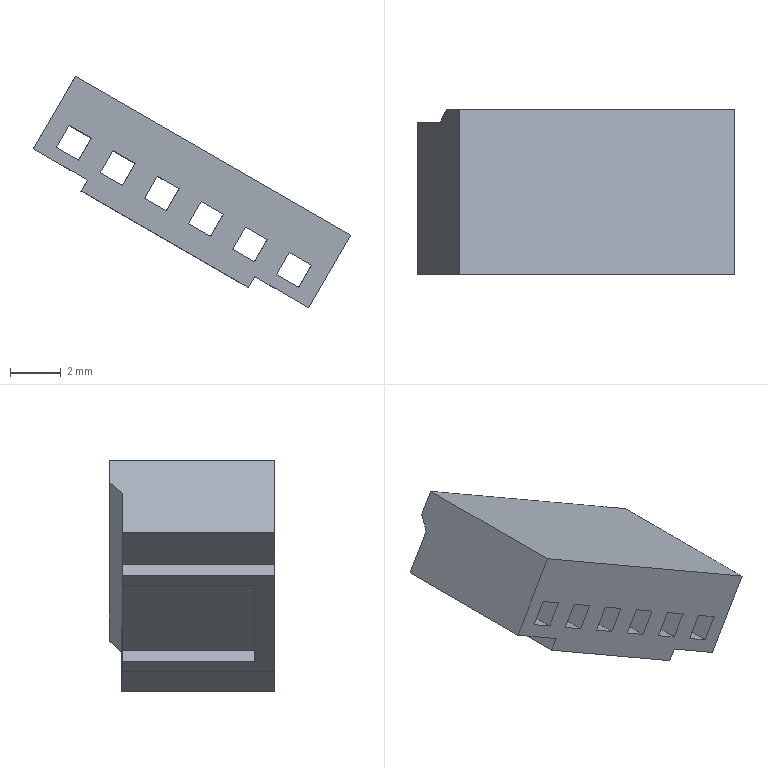Part | SolidWorks | features BaseBody 1 | 1 solid | 40 faces | box 12.481 x 6.512 x 9.108 mm | volume 226.512 mm3 | plane 40
STEP:
#1=CARTESIAN_POINT('',(350.276,384.272,114.82));
#2=VERTEX_POINT('',#1);
#3=CARTESIAN_POINT('',(350.026,384.272,114.387));
#4=VERTEX_POINT('',#3);
#5=CARTESIAN_POINT('',(350.276,384.272,114.82));
#6=DIRECTION('',(-0.5,-0.0004799,-0.866));
#7=VECTOR('',#6,1000.);
#8=LINE('',#5,#7);
#9=EDGE_CURVE('',#2,#4,#8,.T.);
#10=ORIENTED_EDGE('',*,*,#9,.T.);
#11=CARTESIAN_POINT('',(350.031,379.072,114.387));
#12=VERTEX_POINT('',#11);
#13=CARTESIAN_POINT('',(350.031,379.072,114.387));
#14=DIRECTION('',(-0.0009599,1.,0.));
#15=VECTOR('',#14,1000.);
#16=LINE('',#13,#15);
#17=EDGE_CURVE('',#12,#4,#16,.T.);
#18=ORIENTED_EDGE('',*,*,#17,.F.);
#19=CARTESIAN_POINT('',(350.281,379.072,114.82));
#20=VERTEX_POINT('',#19);
#21=CARTESIAN_POINT('',(350.281,379.072,114.82));
#22=DIRECTION('',(-0.5,-0.0004799,-0.866));
#23=VECTOR('',#22,1000.);
#24=LINE('',#21,#23);
#25=EDGE_CURVE('',#20,#12,#24,.T.);
#26=ORIENTED_EDGE('',*,*,#25,.F.);
#27=CARTESIAN_POINT('',(350.281,379.072,114.82));
#28=DIRECTION('',(-0.0009599,1.,0.));
#29=VECTOR('',#28,1000.);
#30=LINE('',#27,#29);
#31=EDGE_CURVE('',#20,#2,#30,.T.);
#32=ORIENTED_EDGE('',*,*,#31,.T.);
#33=EDGE_LOOP('',(#10,#18,#26,#32));
#34=FACE_OUTER_BOUND('',#33,.T.);
#35=CARTESIAN_POINT('',(350.031,378.272,114.387));
#36=DIRECTION('',(-0.866,-0.0008313,0.5));
#37=DIRECTION('',(-0.0009599,1.,0.));
#38=AXIS2_PLACEMENT_3D('',#35,#36,#37);
#39=PLANE('',#38);
#40=ADVANCED_FACE('',(#34),#39,.T.);
#41=ORIENTED_EDGE('',*,*,#25,.T.);
#42=CARTESIAN_POINT('',(344.835,379.067,117.387));
#43=VERTEX_POINT('',#42);
#44=CARTESIAN_POINT('',(344.835,379.067,117.387));
#45=DIRECTION('',(0.866,0.0008313,-0.5));
#46=VECTOR('',#45,1000.);
#47=LINE('',#44,#46);
#48=EDGE_CURVE('',#43,#12,#47,.T.);
#49=ORIENTED_EDGE('',*,*,#48,.F.);
#50=CARTESIAN_POINT('',(345.085,379.067,117.82));
#51=VERTEX_POINT('',#50);
#52=CARTESIAN_POINT('',(345.085,379.067,117.82));
#53=DIRECTION('',(-0.5,-0.0004799,-0.866));
#54=VECTOR('',#53,1000.);
#55=LINE('',#52,#54);
#56=EDGE_CURVE('',#51,#43,#55,.T.);
#57=ORIENTED_EDGE('',*,*,#56,.F.);
#58=CARTESIAN_POINT('',(345.085,379.067,117.82));
#59=DIRECTION('',(0.866,0.0008313,-0.5));
#60=VECTOR('',#59,1000.);
#61=LINE('',#58,#60);
#62=EDGE_CURVE('',#51,#20,#61,.T.);
#63=ORIENTED_EDGE('',*,*,#62,.T.);
#64=EDGE_LOOP('',(#41,#49,#57,#63));
#65=FACE_OUTER_BOUND('',#64,.T.);
#66=CARTESIAN_POINT('',(350.724,379.072,113.987));
#67=DIRECTION('',(-0.0009599,1.,0.));
#68=DIRECTION('',(0.,0.,1.));
#69=AXIS2_PLACEMENT_3D('',#66,#67,#68);
#70=PLANE('',#69);
#71=ADVANCED_FACE('',(#65),#70,.T.);
#72=ORIENTED_EDGE('',*,*,#31,.F.);
#73=ORIENTED_EDGE('',*,*,#62,.F.);
#74=CARTESIAN_POINT('',(345.08,384.267,117.82));
#75=VERTEX_POINT('',#74);
#76=CARTESIAN_POINT('',(345.08,384.267,117.82));
#77=DIRECTION('',(0.0009599,-1.,0.));
#78=VECTOR('',#77,1000.);
#79=LINE('',#76,#78);
#80=EDGE_CURVE('',#75,#51,#79,.T.);
#81=ORIENTED_EDGE('',*,*,#80,.F.);
#82=CARTESIAN_POINT('',(345.08,384.267,117.82));
#83=DIRECTION('',(0.866,0.0008313,-0.5));
#84=VECTOR('',#83,1000.);
#85=LINE('',#82,#84);
#86=EDGE_CURVE('',#75,#2,#85,.T.);
#87=ORIENTED_EDGE('',*,*,#86,.T.);
#88=EDGE_LOOP('',(#72,#73,#81,#87));
#89=FACE_OUTER_BOUND('',#88,.T.);
#90=CARTESIAN_POINT('',(342.265,384.264,119.445));
#91=DIRECTION('',(0.5,0.0004799,0.866));
#92=DIRECTION('',(0.0009599,-1.,0.));
#93=AXIS2_PLACEMENT_3D('',#90,#91,#92);
#94=PLANE('',#93);
#95=ADVANCED_FACE('',(#89),#94,.F.);
#96=ORIENTED_EDGE('',*,*,#56,.T.);
#97=CARTESIAN_POINT('',(344.83,384.267,117.387));
#98=VERTEX_POINT('',#97);
#99=CARTESIAN_POINT('',(344.83,384.267,117.387));
#100=DIRECTION('',(0.0009599,-1.,0.));
#101=VECTOR('',#100,1000.);
#102=LINE('',#99,#101);
#103=EDGE_CURVE('',#98,#43,#102,.T.);
#104=ORIENTED_EDGE('',*,*,#103,.F.);
#105=CARTESIAN_POINT('',(345.08,384.267,117.82));
#106=DIRECTION('',(-0.5,-0.0004799,-0.866));
#107=VECTOR('',#106,1000.);
#108=LINE('',#105,#107);
#109=EDGE_CURVE('',#75,#98,#108,.T.);
#110=ORIENTED_EDGE('',*,*,#109,.F.);
#111=ORIENTED_EDGE('',*,*,#80,.T.);
#112=EDGE_LOOP('',(#96,#104,#110,#111));
#113=FACE_OUTER_BOUND('',#112,.T.);
#114=CARTESIAN_POINT('',(344.835,378.267,117.387));
#115=DIRECTION('',(0.866,0.0008313,-0.5));
#116=DIRECTION('',(0.,-1.,-0.001663));
#117=AXIS2_PLACEMENT_3D('',#114,#115,#116);
#118=PLANE('',#117);
#119=ADVANCED_FACE('',(#113),#118,.T.);
#120=CARTESIAN_POINT('',(350.974,378.273,114.42));
#121=VERTEX_POINT('',#120);
#122=CARTESIAN_POINT('',(350.724,378.272,113.987));
#123=VERTEX_POINT('',#122);
#124=CARTESIAN_POINT('',(350.974,378.273,114.42));
#125=DIRECTION('',(-0.5,-0.0004799,-0.866));
#126=VECTOR('',#125,1000.);
#127=LINE('',#124,#126);
#128=EDGE_CURVE('',#121,#123,#127,.T.);
#129=ORIENTED_EDGE('',*,*,#128,.T.);
#130=CARTESIAN_POINT('',(350.719,384.272,113.987));
#131=VERTEX_POINT('',#130);
#132=CARTESIAN_POINT('',(350.724,378.272,113.987));
#133=DIRECTION('',(-0.0009599,1.,0.));
#134=VECTOR('',#133,1000.);
#135=LINE('',#132,#134);
#136=EDGE_CURVE('',#123,#131,#135,.T.);
#137=ORIENTED_EDGE('',*,*,#136,.T.);
#138=CARTESIAN_POINT('',(350.969,384.273,114.42));
#139=VERTEX_POINT('',#138);
#140=CARTESIAN_POINT('',(350.969,384.273,114.42));
#141=DIRECTION('',(-0.5,-0.0004799,-0.866));
#142=VECTOR('',#141,1000.);
#143=LINE('',#140,#142);
#144=EDGE_CURVE('',#139,#131,#143,.T.);
#145=ORIENTED_EDGE('',*,*,#144,.F.);
#146=CARTESIAN_POINT('',(350.974,378.273,114.42));
#147=DIRECTION('',(-0.0009599,1.,0.));
#148=VECTOR('',#147,1000.);
#149=LINE('',#146,#148);
#150=EDGE_CURVE('',#121,#139,#149,.T.);
#151=ORIENTED_EDGE('',*,*,#150,.F.);
#152=EDGE_LOOP('',(#129,#137,#145,#151));
#153=FACE_OUTER_BOUND('',#152,.T.);
#154=CARTESIAN_POINT('',(350.724,378.272,113.987));
#155=DIRECTION('',(-0.866,-0.0008313,0.5));
#156=DIRECTION('',(-0.0009599,1.,0.));
#157=AXIS2_PLACEMENT_3D('',#154,#155,#156);
#158=PLANE('',#157);
#159=ADVANCED_FACE('',(#153),#158,.F.);
#160=CARTESIAN_POINT('',(353.09,384.275,113.195));
#161=VERTEX_POINT('',#160);
#162=CARTESIAN_POINT('',(350.969,384.273,114.42));
#163=DIRECTION('',(0.866,0.0008313,-0.5));
#164=VECTOR('',#163,1000.);
#165=LINE('',#162,#164);
#166=EDGE_CURVE('',#139,#161,#165,.T.);
#167=ORIENTED_EDGE('',*,*,#166,.T.);
#168=CARTESIAN_POINT('',(353.096,378.275,113.195));
#169=VERTEX_POINT('',#168);
#170=CARTESIAN_POINT('',(353.096,378.275,113.195));
#171=DIRECTION('',(-0.0009599,1.,0.));
#172=VECTOR('',#171,1000.);
#173=LINE('',#170,#172);
#174=EDGE_CURVE('',#169,#161,#173,.T.);
#175=ORIENTED_EDGE('',*,*,#174,.F.);
#176=CARTESIAN_POINT('',(350.974,378.273,114.42));
#177=DIRECTION('',(0.866,0.0008313,-0.5));
#178=VECTOR('',#177,1000.);
#179=LINE('',#176,#178);
#180=EDGE_CURVE('',#121,#169,#179,.T.);
#181=ORIENTED_EDGE('',*,*,#180,.F.);
#182=ORIENTED_EDGE('',*,*,#150,.T.);
#183=EDGE_LOOP('',(#167,#175,#181,#182));
#184=FACE_OUTER_BOUND('',#183,.T.);
#185=CARTESIAN_POINT('',(342.265,384.264,119.445));
#186=DIRECTION('',(0.5,0.0004799,0.866));
#187=DIRECTION('',(0.0009599,-1.,0.));
#188=AXIS2_PLACEMENT_3D('',#185,#186,#187);
#189=PLANE('',#188);
#190=ADVANCED_FACE('',(#184),#189,.F.);
#191=CARTESIAN_POINT('',(354.74,384.776,116.053));
#192=VERTEX_POINT('',#191);
#193=CARTESIAN_POINT('',(343.914,384.766,122.303));
#194=VERTEX_POINT('',#193);
#195=CARTESIAN_POINT('',(354.74,384.776,116.053));
#196=DIRECTION('',(-0.866,-0.0008313,0.5));
#197=VECTOR('',#196,1000.);
#198=LINE('',#195,#197);
#199=EDGE_CURVE('',#192,#194,#198,.T.);
#200=ORIENTED_EDGE('',*,*,#199,.F.);
#201=CARTESIAN_POINT('',(354.24,384.776,115.187));
#202=VERTEX_POINT('',#201);
#203=CARTESIAN_POINT('',(354.24,384.776,115.187));
#204=DIRECTION('',(0.5,0.0004799,0.866));
#205=VECTOR('',#204,1000.);
#206=LINE('',#203,#205);
#207=EDGE_CURVE('',#202,#192,#206,.T.);
#208=ORIENTED_EDGE('',*,*,#207,.F.);
#209=CARTESIAN_POINT('',(343.414,384.765,121.437));
#210=VERTEX_POINT('',#209);
#211=CARTESIAN_POINT('',(343.414,384.765,121.437));
#212=DIRECTION('',(0.866,0.0008313,-0.5));
#213=VECTOR('',#212,1000.);
#214=LINE('',#211,#213);
#215=EDGE_CURVE('',#210,#202,#214,.T.);
#216=ORIENTED_EDGE('',*,*,#215,.F.);
#217=CARTESIAN_POINT('',(343.914,384.766,122.303));
#218=DIRECTION('',(-0.5,-0.0004799,-0.866));
#219=VECTOR('',#218,1000.);
#220=LINE('',#217,#219);
#221=EDGE_CURVE('',#194,#210,#220,.T.);
#222=ORIENTED_EDGE('',*,*,#221,.F.);
#223=EDGE_LOOP('',(#200,#208,#216,#222));
#224=FACE_OUTER_BOUND('',#223,.T.);
#225=CARTESIAN_POINT('',(348.502,384.77,117.749));
#226=DIRECTION('',(0.0009599,-1.,0.));
#227=DIRECTION('',(0.,0.,-1.));
#228=AXIS2_PLACEMENT_3D('',#225,#226,#227);
#229=PLANE('',#228);
#230=ADVANCED_FACE('',(#224),#229,.F.);
#231=CARTESIAN_POINT('',(353.99,384.276,114.754));
#232=VERTEX_POINT('',#231);
#233=CARTESIAN_POINT('',(343.165,384.265,121.004));
#234=VERTEX_POINT('',#233);
#235=CARTESIAN_POINT('',(353.99,384.276,114.754));
#236=DIRECTION('',(-0.866,-0.0008313,0.5));
#237=VECTOR('',#236,1000.);
#238=LINE('',#235,#237);
#239=EDGE_CURVE('',#232,#234,#238,.T.);
#240=ORIENTED_EDGE('',*,*,#239,.T.);
#241=CARTESIAN_POINT('',(343.414,384.765,121.437));
#242=DIRECTION('',(-0.3529,-0.7074,-0.6124));
#243=VECTOR('',#242,1000.);
#244=LINE('',#241,#243);
#245=EDGE_CURVE('',#210,#234,#244,.T.);
#246=ORIENTED_EDGE('',*,*,#245,.F.);
#247=ORIENTED_EDGE('',*,*,#215,.T.);
#248=CARTESIAN_POINT('',(353.99,384.276,114.754));
#249=DIRECTION('',(0.3529,0.7074,0.6124));
#250=VECTOR('',#249,1000.);
#251=LINE('',#248,#250);
#252=EDGE_CURVE('',#232,#202,#251,.T.);
#253=ORIENTED_EDGE('',*,*,#252,.F.);
#254=EDGE_LOOP('',(#240,#246,#247,#253));
#255=FACE_OUTER_BOUND('',#254,.T.);
#256=CARTESIAN_POINT('',(343.414,384.765,121.437));
#257=DIRECTION('',(-0.3542,0.7068,-0.6124));
#258=DIRECTION('',(-0.8656,0.,0.5007));
#259=AXIS2_PLACEMENT_3D('',#256,#257,#258);
#260=PLANE('',#259);
#261=ADVANCED_FACE('',(#255),#260,.T.);
#262=CARTESIAN_POINT('',(343.921,378.266,122.303));
#263=VERTEX_POINT('',#262);
#264=CARTESIAN_POINT('',(343.921,378.266,122.303));
#265=DIRECTION('',(-0.0009599,1.,0.));
#266=VECTOR('',#265,1000.);
#267=LINE('',#264,#266);
#268=EDGE_CURVE('',#263,#194,#267,.T.);
#269=ORIENTED_EDGE('',*,*,#268,.T.);
#270=ORIENTED_EDGE('',*,*,#221,.T.);
#271=ORIENTED_EDGE('',*,*,#245,.T.);
#272=CARTESIAN_POINT('',(342.265,384.264,119.445));
#273=VERTEX_POINT('',#272);
#274=CARTESIAN_POINT('',(343.165,384.265,121.004));
#275=DIRECTION('',(-0.5,-0.0004799,-0.866));
#276=VECTOR('',#275,1000.);
#277=LINE('',#274,#276);
#278=EDGE_CURVE('',#234,#273,#277,.T.);
#279=ORIENTED_EDGE('',*,*,#278,.T.);
#280=CARTESIAN_POINT('',(342.271,378.264,119.445));
#281=VERTEX_POINT('',#280);
#282=CARTESIAN_POINT('',(342.271,378.264,119.445));
#283=DIRECTION('',(-0.0009599,1.,0.));
#284=VECTOR('',#283,1000.);
#285=LINE('',#282,#284);
#286=EDGE_CURVE('',#281,#273,#285,.T.);
#287=ORIENTED_EDGE('',*,*,#286,.F.);
#288=CARTESIAN_POINT('',(343.921,378.266,122.303));
#289=DIRECTION('',(-0.5,-0.0004799,-0.866));
#290=VECTOR('',#289,1000.);
#291=LINE('',#288,#290);
#292=EDGE_CURVE('',#263,#281,#291,.T.);
#293=ORIENTED_EDGE('',*,*,#292,.F.);
#294=EDGE_LOOP('',(#269,#270,#271,#279,#287,#293));
#295=FACE_OUTER_BOUND('',#294,.T.);
#296=CARTESIAN_POINT('',(343.915,384.266,122.303));
#297=DIRECTION('',(0.866,0.0008313,-0.5));
#298=DIRECTION('',(0.,-1.,-0.001663));
#299=AXIS2_PLACEMENT_3D('',#296,#297,#298);
#300=PLANE('',#299);
#301=ADVANCED_FACE('',(#295),#300,.F.);
#302=CARTESIAN_POINT('',(354.746,378.276,116.053));
#303=VERTEX_POINT('',#302);
#304=CARTESIAN_POINT('',(354.746,378.276,116.053));
#305=DIRECTION('',(-0.0009599,1.,0.));
#306=VECTOR('',#305,1000.);
#307=LINE('',#304,#306);
#308=EDGE_CURVE('',#303,#192,#307,.T.);
#309=ORIENTED_EDGE('',*,*,#308,.T.);
#310=ORIENTED_EDGE('',*,*,#199,.T.);
#311=ORIENTED_EDGE('',*,*,#268,.F.);
#312=CARTESIAN_POINT('',(354.746,378.276,116.053));
#313=DIRECTION('',(-0.866,-0.0008313,0.5));
#314=VECTOR('',#313,1000.);
#315=LINE('',#312,#314);
#316=EDGE_CURVE('',#303,#263,#315,.T.);
#317=ORIENTED_EDGE('',*,*,#316,.F.);
#318=EDGE_LOOP('',(#309,#310,#311,#317));
#319=FACE_OUTER_BOUND('',#318,.T.);
#320=CARTESIAN_POINT('',(343.915,384.266,122.303));
#321=DIRECTION('',(-0.5,-0.0004799,-0.866));
#322=DIRECTION('',(-0.866,0.,0.5));
#323=AXIS2_PLACEMENT_3D('',#320,#321,#322);
#324=PLANE('',#323);
#325=ADVANCED_FACE('',(#319),#324,.F.);
#326=ORIENTED_EDGE('',*,*,#174,.T.);
#327=CARTESIAN_POINT('',(353.09,384.275,113.195));
#328=DIRECTION('',(0.5,0.0004799,0.866));
#329=VECTOR('',#328,1000.);
#330=LINE('',#327,#329);
#331=EDGE_CURVE('',#161,#232,#330,.T.);
#332=ORIENTED_EDGE('',*,*,#331,.T.);
#333=ORIENTED_EDGE('',*,*,#252,.T.);
#334=ORIENTED_EDGE('',*,*,#207,.T.);
#335=ORIENTED_EDGE('',*,*,#308,.F.);
#336=CARTESIAN_POINT('',(353.096,378.275,113.195));
#337=DIRECTION('',(0.5,0.0004799,0.866));
#338=VECTOR('',#337,1000.);
#339=LINE('',#336,#338);
#340=EDGE_CURVE('',#169,#303,#339,.T.);
#341=ORIENTED_EDGE('',*,*,#340,.F.);
#342=EDGE_LOOP('',(#326,#332,#333,#334,#335,#341));
#343=FACE_OUTER_BOUND('',#342,.T.);
#344=CARTESIAN_POINT('',(354.74,384.276,116.053));
#345=DIRECTION('',(-0.866,-0.0008313,0.5));
#346=DIRECTION('',(-0.0009599,1.,0.));
#347=AXIS2_PLACEMENT_3D('',#344,#345,#346);
#348=PLANE('',#347);
#349=ADVANCED_FACE('',(#343),#348,.F.);
#350=CARTESIAN_POINT('',(346.634,378.269,117.503));
#351=VERTEX_POINT('',#350);
#352=CARTESIAN_POINT('',(346.629,384.269,117.503));
#353=VERTEX_POINT('',#352);
#354=CARTESIAN_POINT('',(346.634,378.269,117.503));
#355=DIRECTION('',(-0.0009599,1.,0.));
#356=VECTOR('',#355,1000.);
#357=LINE('',#354,#356);
#358=EDGE_CURVE('',#351,#353,#357,.T.);
#359=ORIENTED_EDGE('',*,*,#358,.T.);
#360=CARTESIAN_POINT('',(347.129,384.269,118.369));
#361=VERTEX_POINT('',#360);
#362=CARTESIAN_POINT('',(347.129,384.269,118.369));
#363=DIRECTION('',(-0.5,-0.0004799,-0.866));
#364=VECTOR('',#363,1000.);
#365=LINE('',#362,#364);
#366=EDGE_CURVE('',#361,#353,#365,.T.);
#367=ORIENTED_EDGE('',*,*,#366,.F.);
#368=CARTESIAN_POINT('',(347.134,378.269,118.369));
#369=VERTEX_POINT('',#368);
#370=CARTESIAN_POINT('',(347.134,378.269,118.369));
#371=DIRECTION('',(-0.0009599,1.,0.));
#372=VECTOR('',#371,1000.);
#373=LINE('',#370,#372);
#374=EDGE_CURVE('',#369,#361,#373,.T.);
#375=ORIENTED_EDGE('',*,*,#374,.F.);
#376=CARTESIAN_POINT('',(347.134,378.269,118.369));
#377=DIRECTION('',(-0.5,-0.0004799,-0.866));
#378=VECTOR('',#377,1000.);
#379=LINE('',#376,#378);
#380=EDGE_CURVE('',#369,#351,#379,.T.);
#381=ORIENTED_EDGE('',*,*,#380,.T.);
#382=EDGE_LOOP('',(#359,#367,#375,#381));
#383=FACE_OUTER_BOUND('',#382,.T.);
#384=CARTESIAN_POINT('',(346.629,384.269,117.503));
#385=DIRECTION('',(0.866,0.0008313,-0.5));
#386=DIRECTION('',(0.,-1.,-0.001663));
#387=AXIS2_PLACEMENT_3D('',#384,#385,#386);
#388=PLANE('',#387);
#389=ADVANCED_FACE('',(#383),#388,.T.);
#390=CARTESIAN_POINT('',(347.5,378.269,117.003));
#391=VERTEX_POINT('',#390);
#392=CARTESIAN_POINT('',(347.495,384.269,117.003));
#393=VERTEX_POINT('',#392);
#394=CARTESIAN_POINT('',(347.5,378.269,117.003));
#395=DIRECTION('',(-0.0009599,1.,0.));
#396=VECTOR('',#395,1000.);
#397=LINE('',#394,#396);
#398=EDGE_CURVE('',#391,#393,#397,.T.);
#399=ORIENTED_EDGE('',*,*,#398,.T.);
#400=CARTESIAN_POINT('',(346.629,384.269,117.503));
#401=DIRECTION('',(0.866,0.0008313,-0.5));
#402=VECTOR('',#401,1000.);
#403=LINE('',#400,#402);
#404=EDGE_CURVE('',#353,#393,#403,.T.);
#405=ORIENTED_EDGE('',*,*,#404,.F.);
#406=ORIENTED_EDGE('',*,*,#358,.F.);
#407=CARTESIAN_POINT('',(346.634,378.269,117.503));
#408=DIRECTION('',(0.866,0.0008313,-0.5));
#409=VECTOR('',#408,1000.);
#410=LINE('',#407,#409);
#411=EDGE_CURVE('',#351,#391,#410,.T.);
#412=ORIENTED_EDGE('',*,*,#411,.T.);
#413=EDGE_LOOP('',(#399,#405,#406,#412));
#414=FACE_OUTER_BOUND('',#413,.T.);
#415=CARTESIAN_POINT('',(347.495,384.269,117.003));
#416=DIRECTION('',(0.5,0.0004799,0.866));
#417=DIRECTION('',(0.0009599,-1.,0.));
#418=AXIS2_PLACEMENT_3D('',#415,#416,#417);
#419=PLANE('',#418);
#420=ADVANCED_FACE('',(#414),#419,.T.);
#421=CARTESIAN_POINT('',(348.,378.27,117.869));
#422=VERTEX_POINT('',#421);
#423=CARTESIAN_POINT('',(347.995,384.27,117.869));
#424=VERTEX_POINT('',#423);
#425=CARTESIAN_POINT('',(348.,378.27,117.869));
#426=DIRECTION('',(-0.0009599,1.,0.));
#427=VECTOR('',#426,1000.);
#428=LINE('',#425,#427);
#429=EDGE_CURVE('',#422,#424,#428,.T.);
#430=ORIENTED_EDGE('',*,*,#429,.T.);
#431=CARTESIAN_POINT('',(347.495,384.269,117.003));
#432=DIRECTION('',(0.5,0.0004799,0.866));
#433=VECTOR('',#432,1000.);
#434=LINE('',#431,#433);
#435=EDGE_CURVE('',#393,#424,#434,.T.);
#436=ORIENTED_EDGE('',*,*,#435,.F.);
#437=ORIENTED_EDGE('',*,*,#398,.F.);
#438=CARTESIAN_POINT('',(347.5,378.269,117.003));
#439=DIRECTION('',(0.5,0.0004799,0.866));
#440=VECTOR('',#439,1000.);
#441=LINE('',#438,#440);
#442=EDGE_CURVE('',#391,#422,#441,.T.);
#443=ORIENTED_EDGE('',*,*,#442,.T.);
#444=EDGE_LOOP('',(#430,#436,#437,#443));
#445=FACE_OUTER_BOUND('',#444,.T.);
#446=CARTESIAN_POINT('',(347.995,384.27,117.869));
#447=DIRECTION('',(-0.866,-0.0008313,0.5));
#448=DIRECTION('',(-0.0009599,1.,0.));
#449=AXIS2_PLACEMENT_3D('',#446,#447,#448);
#450=PLANE('',#449);
#451=ADVANCED_FACE('',(#445),#450,.T.);
#452=ORIENTED_EDGE('',*,*,#374,.T.);
#453=CARTESIAN_POINT('',(347.995,384.27,117.869));
#454=DIRECTION('',(-0.866,-0.0008313,0.5));
#455=VECTOR('',#454,1000.);
#456=LINE('',#453,#455);
#457=EDGE_CURVE('',#424,#361,#456,.T.);
#458=ORIENTED_EDGE('',*,*,#457,.F.);
#459=ORIENTED_EDGE('',*,*,#429,.F.);
#460=CARTESIAN_POINT('',(348.,378.27,117.869));
#461=DIRECTION('',(-0.866,-0.0008313,0.5));
#462=VECTOR('',#461,1000.);
#463=LINE('',#460,#462);
#464=EDGE_CURVE('',#422,#369,#463,.T.);
#465=ORIENTED_EDGE('',*,*,#464,.T.);
#466=EDGE_LOOP('',(#452,#458,#459,#465));
#467=FACE_OUTER_BOUND('',#466,.T.);
#468=CARTESIAN_POINT('',(347.129,384.269,118.369));
#469=DIRECTION('',(-0.5,-0.0004799,-0.866));
#470=DIRECTION('',(-0.866,0.,0.5));
#471=AXIS2_PLACEMENT_3D('',#468,#469,#470);
#472=PLANE('',#471);
#473=ADVANCED_FACE('',(#467),#472,.T.);
#474=CARTESIAN_POINT('',(344.902,378.267,118.503));
#475=VERTEX_POINT('',#474);
#476=CARTESIAN_POINT('',(344.897,384.267,118.503));
#477=VERTEX_POINT('',#476);
#478=CARTESIAN_POINT('',(344.902,378.267,118.503));
#479=DIRECTION('',(-0.0009599,1.,0.));
#480=VECTOR('',#479,1000.);
#481=LINE('',#478,#480);
#482=EDGE_CURVE('',#475,#477,#481,.T.);
#483=ORIENTED_EDGE('',*,*,#482,.T.);
#484=CARTESIAN_POINT('',(345.397,384.267,119.369));
#485=VERTEX_POINT('',#484);
#486=CARTESIAN_POINT('',(345.397,384.267,119.369));
#487=DIRECTION('',(-0.5,-0.0004799,-0.866));
#488=VECTOR('',#487,1000.);
#489=LINE('',#486,#488);
#490=EDGE_CURVE('',#485,#477,#489,.T.);
#491=ORIENTED_EDGE('',*,*,#490,.F.);
#492=CARTESIAN_POINT('',(345.402,378.267,119.369));
#493=VERTEX_POINT('',#492);
#494=CARTESIAN_POINT('',(345.402,378.267,119.369));
#495=DIRECTION('',(-0.0009599,1.,0.));
#496=VECTOR('',#495,1000.);
#497=LINE('',#494,#496);
#498=EDGE_CURVE('',#493,#485,#497,.T.);
#499=ORIENTED_EDGE('',*,*,#498,.F.);
#500=CARTESIAN_POINT('',(345.402,378.267,119.369));
#501=DIRECTION('',(-0.5,-0.0004799,-0.866));
#502=VECTOR('',#501,1000.);
#503=LINE('',#500,#502);
#504=EDGE_CURVE('',#493,#475,#503,.T.);
#505=ORIENTED_EDGE('',*,*,#504,.T.);
#506=EDGE_LOOP('',(#483,#491,#499,#505));
#507=FACE_OUTER_BOUND('',#506,.T.);
#508=CARTESIAN_POINT('',(344.897,384.267,118.503));
#509=DIRECTION('',(0.866,0.0008313,-0.5));
#510=DIRECTION('',(0.,-1.,-0.001663));
#511=AXIS2_PLACEMENT_3D('',#508,#509,#510);
#512=PLANE('',#511);
#513=ADVANCED_FACE('',(#507),#512,.T.);
#514=CARTESIAN_POINT('',(345.768,378.268,118.003));
#515=VERTEX_POINT('',#514);
#516=CARTESIAN_POINT('',(345.763,384.268,118.003));
#517=VERTEX_POINT('',#516);
#518=CARTESIAN_POINT('',(345.768,378.268,118.003));
#519=DIRECTION('',(-0.0009599,1.,0.));
#520=VECTOR('',#519,1000.);
#521=LINE('',#518,#520);
#522=EDGE_CURVE('',#515,#517,#521,.T.);
#523=ORIENTED_EDGE('',*,*,#522,.T.);
#524=CARTESIAN_POINT('',(344.897,384.267,118.503));
#525=DIRECTION('',(0.866,0.0008313,-0.5));
#526=VECTOR('',#525,1000.);
#527=LINE('',#524,#526);
#528=EDGE_CURVE('',#477,#517,#527,.T.);
#529=ORIENTED_EDGE('',*,*,#528,.F.);
#530=ORIENTED_EDGE('',*,*,#482,.F.);
#531=CARTESIAN_POINT('',(344.902,378.267,118.503));
#532=DIRECTION('',(0.866,0.0008313,-0.5));
#533=VECTOR('',#532,1000.);
#534=LINE('',#531,#533);
#535=EDGE_CURVE('',#475,#515,#534,.T.);
#536=ORIENTED_EDGE('',*,*,#535,.T.);
#537=EDGE_LOOP('',(#523,#529,#530,#536));
#538=FACE_OUTER_BOUND('',#537,.T.);
#539=CARTESIAN_POINT('',(345.763,384.268,118.003));
#540=DIRECTION('',(0.5,0.0004799,0.866));
#541=DIRECTION('',(0.0009599,-1.,0.));
#542=AXIS2_PLACEMENT_3D('',#539,#540,#541);
#543=PLANE('',#542);
#544=ADVANCED_FACE('',(#538),#543,.T.);
#545=CARTESIAN_POINT('',(346.268,378.268,118.869));
#546=VERTEX_POINT('',#545);
#547=CARTESIAN_POINT('',(346.263,384.268,118.869));
#548=VERTEX_POINT('',#547);
#549=CARTESIAN_POINT('',(346.268,378.268,118.869));
#550=DIRECTION('',(-0.0009599,1.,0.));
#551=VECTOR('',#550,1000.);
#552=LINE('',#549,#551);
#553=EDGE_CURVE('',#546,#548,#552,.T.);
#554=ORIENTED_EDGE('',*,*,#553,.T.);
#555=CARTESIAN_POINT('',(345.763,384.268,118.003));
#556=DIRECTION('',(0.5,0.0004799,0.866));
#557=VECTOR('',#556,1000.);
#558=LINE('',#555,#557);
#559=EDGE_CURVE('',#517,#548,#558,.T.);
#560=ORIENTED_EDGE('',*,*,#559,.F.);
#561=ORIENTED_EDGE('',*,*,#522,.F.);
#562=CARTESIAN_POINT('',(345.768,378.268,118.003));
#563=DIRECTION('',(0.5,0.0004799,0.866));
#564=VECTOR('',#563,1000.);
#565=LINE('',#562,#564);
#566=EDGE_CURVE('',#515,#546,#565,.T.);
#567=ORIENTED_EDGE('',*,*,#566,.T.);
#568=EDGE_LOOP('',(#554,#560,#561,#567));
#569=FACE_OUTER_BOUND('',#568,.T.);
#570=CARTESIAN_POINT('',(346.263,384.268,118.869));
#571=DIRECTION('',(-0.866,-0.0008313,0.5));
#572=DIRECTION('',(-0.0009599,1.,0.));
#573=AXIS2_PLACEMENT_3D('',#570,#571,#572);
#574=PLANE('',#573);
#575=ADVANCED_FACE('',(#569),#574,.T.);
#576=ORIENTED_EDGE('',*,*,#498,.T.);
#577=CARTESIAN_POINT('',(346.263,384.268,118.869));
#578=DIRECTION('',(-0.866,-0.0008313,0.5));
#579=VECTOR('',#578,1000.);
#580=LINE('',#577,#579);
#581=EDGE_CURVE('',#548,#485,#580,.T.);
#582=ORIENTED_EDGE('',*,*,#581,.F.);
#583=ORIENTED_EDGE('',*,*,#553,.F.);
#584=CARTESIAN_POINT('',(346.268,378.268,118.869));
#585=DIRECTION('',(-0.866,-0.0008313,0.5));
#586=VECTOR('',#585,1000.);
#587=LINE('',#584,#586);
#588=EDGE_CURVE('',#546,#493,#587,.T.);
#589=ORIENTED_EDGE('',*,*,#588,.T.);
#590=EDGE_LOOP('',(#576,#582,#583,#589));
#591=FACE_OUTER_BOUND('',#590,.T.);
#592=CARTESIAN_POINT('',(345.397,384.267,119.369));
#593=DIRECTION('',(-0.5,-0.0004799,-0.866));
#594=DIRECTION('',(-0.866,0.,0.5));
#595=AXIS2_PLACEMENT_3D('',#592,#593,#594);
#596=PLANE('',#595);
#597=ADVANCED_FACE('',(#591),#596,.T.);
#598=CARTESIAN_POINT('',(343.17,378.265,119.503));
#599=VERTEX_POINT('',#598);
#600=CARTESIAN_POINT('',(343.164,384.265,119.503));
#601=VERTEX_POINT('',#600);
#602=CARTESIAN_POINT('',(343.17,378.265,119.503));
#603=DIRECTION('',(-0.0009599,1.,0.));
#604=VECTOR('',#603,1000.);
#605=LINE('',#602,#604);
#606=EDGE_CURVE('',#599,#601,#605,.T.);
#607=ORIENTED_EDGE('',*,*,#606,.T.);
#608=CARTESIAN_POINT('',(343.664,384.266,120.369));
#609=VERTEX_POINT('',#608);
#610=CARTESIAN_POINT('',(343.664,384.266,120.369));
#611=DIRECTION('',(-0.5,-0.0004799,-0.866));
#612=VECTOR('',#611,1000.);
#613=LINE('',#610,#612);
#614=EDGE_CURVE('',#609,#601,#613,.T.);
#615=ORIENTED_EDGE('',*,*,#614,.F.);
#616=CARTESIAN_POINT('',(343.67,378.266,120.369));
#617=VERTEX_POINT('',#616);
#618=CARTESIAN_POINT('',(343.67,378.266,120.369));
#619=DIRECTION('',(-0.0009599,1.,0.));
#620=VECTOR('',#619,1000.);
#621=LINE('',#618,#620);
#622=EDGE_CURVE('',#617,#609,#621,.T.);
#623=ORIENTED_EDGE('',*,*,#622,.F.);
#624=CARTESIAN_POINT('',(343.67,378.266,120.369));
#625=DIRECTION('',(-0.5,-0.0004799,-0.866));
#626=VECTOR('',#625,1000.);
#627=LINE('',#624,#626);
#628=EDGE_CURVE('',#617,#599,#627,.T.);
#629=ORIENTED_EDGE('',*,*,#628,.T.);
#630=EDGE_LOOP('',(#607,#615,#623,#629));
#631=FACE_OUTER_BOUND('',#630,.T.);
#632=CARTESIAN_POINT('',(343.164,384.265,119.503));
#633=DIRECTION('',(0.866,0.0008313,-0.5));
#634=DIRECTION('',(0.,-1.,-0.001663));
#635=AXIS2_PLACEMENT_3D('',#632,#633,#634);
#636=PLANE('',#635);
#637=ADVANCED_FACE('',(#631),#636,.T.);
#638=CARTESIAN_POINT('',(344.036,378.266,119.003));
#639=VERTEX_POINT('',#638);
#640=CARTESIAN_POINT('',(344.031,384.266,119.003));
#641=VERTEX_POINT('',#640);
#642=CARTESIAN_POINT('',(344.036,378.266,119.003));
#643=DIRECTION('',(-0.0009599,1.,0.));
#644=VECTOR('',#643,1000.);
#645=LINE('',#642,#644);
#646=EDGE_CURVE('',#639,#641,#645,.T.);
#647=ORIENTED_EDGE('',*,*,#646,.T.);
#648=CARTESIAN_POINT('',(343.164,384.265,119.503));
#649=DIRECTION('',(0.866,0.0008313,-0.5));
#650=VECTOR('',#649,1000.);
#651=LINE('',#648,#650);
#652=EDGE_CURVE('',#601,#641,#651,.T.);
#653=ORIENTED_EDGE('',*,*,#652,.F.);
#654=ORIENTED_EDGE('',*,*,#606,.F.);
#655=CARTESIAN_POINT('',(343.17,378.265,119.503));
#656=DIRECTION('',(0.866,0.0008313,-0.5));
#657=VECTOR('',#656,1000.);
#658=LINE('',#655,#657);
#659=EDGE_CURVE('',#599,#639,#658,.T.);
#660=ORIENTED_EDGE('',*,*,#659,.T.);
#661=EDGE_LOOP('',(#647,#653,#654,#660));
#662=FACE_OUTER_BOUND('',#661,.T.);
#663=CARTESIAN_POINT('',(344.031,384.266,119.003));
#664=DIRECTION('',(0.5,0.0004799,0.866));
#665=DIRECTION('',(0.0009599,-1.,0.));
#666=AXIS2_PLACEMENT_3D('',#663,#664,#665);
#667=PLANE('',#666);
#668=ADVANCED_FACE('',(#662),#667,.T.);
#669=CARTESIAN_POINT('',(344.536,378.267,119.869));
#670=VERTEX_POINT('',#669);
#671=CARTESIAN_POINT('',(344.531,384.267,119.869));
#672=VERTEX_POINT('',#671);
#673=CARTESIAN_POINT('',(344.536,378.267,119.869));
#674=DIRECTION('',(-0.0009599,1.,0.));
#675=VECTOR('',#674,1000.);
#676=LINE('',#673,#675);
#677=EDGE_CURVE('',#670,#672,#676,.T.);
#678=ORIENTED_EDGE('',*,*,#677,.T.);
#679=CARTESIAN_POINT('',(344.031,384.266,119.003));
#680=DIRECTION('',(0.5,0.0004799,0.866));
#681=VECTOR('',#680,1000.);
#682=LINE('',#679,#681);
#683=EDGE_CURVE('',#641,#672,#682,.T.);
#684=ORIENTED_EDGE('',*,*,#683,.F.);
#685=ORIENTED_EDGE('',*,*,#646,.F.);
#686=CARTESIAN_POINT('',(344.036,378.266,119.003));
#687=DIRECTION('',(0.5,0.0004799,0.866));
#688=VECTOR('',#687,1000.);
#689=LINE('',#686,#688);
#690=EDGE_CURVE('',#639,#670,#689,.T.);
#691=ORIENTED_EDGE('',*,*,#690,.T.);
#692=EDGE_LOOP('',(#678,#684,#685,#691));
#693=FACE_OUTER_BOUND('',#692,.T.);
#694=CARTESIAN_POINT('',(344.531,384.267,119.869));
#695=DIRECTION('',(-0.866,-0.0008313,0.5));
#696=DIRECTION('',(-0.0009599,1.,0.));
#697=AXIS2_PLACEMENT_3D('',#694,#695,#696);
#698=PLANE('',#697);
#699=ADVANCED_FACE('',(#693),#698,.T.);
#700=ORIENTED_EDGE('',*,*,#622,.T.);
#701=CARTESIAN_POINT('',(344.531,384.267,119.869));
#702=DIRECTION('',(-0.866,-0.0008313,0.5));
#703=VECTOR('',#702,1000.);
#704=LINE('',#701,#703);
#705=EDGE_CURVE('',#672,#609,#704,.T.);
#706=ORIENTED_EDGE('',*,*,#705,.F.);
#707=ORIENTED_EDGE('',*,*,#677,.F.);
#708=CARTESIAN_POINT('',(344.536,378.267,119.869));
#709=DIRECTION('',(-0.866,-0.0008313,0.5));
#710=VECTOR('',#709,1000.);
#711=LINE('',#708,#710);
#712=EDGE_CURVE('',#670,#617,#711,.T.);
#713=ORIENTED_EDGE('',*,*,#712,.T.);
#714=EDGE_LOOP('',(#700,#706,#707,#713));
#715=FACE_OUTER_BOUND('',#714,.T.);
#716=CARTESIAN_POINT('',(343.664,384.266,120.369));
#717=DIRECTION('',(-0.5,-0.0004799,-0.866));
#718=DIRECTION('',(-0.866,0.,0.5));
#719=AXIS2_PLACEMENT_3D('',#716,#717,#718);
#720=PLANE('',#719);
#721=ADVANCED_FACE('',(#715),#720,.T.);
#722=CARTESIAN_POINT('',(352.697,378.274,114.003));
#723=VERTEX_POINT('',#722);
#724=CARTESIAN_POINT('',(352.691,384.274,114.003));
#725=VERTEX_POINT('',#724);
#726=CARTESIAN_POINT('',(352.697,378.274,114.003));
#727=DIRECTION('',(-0.0009599,1.,0.));
#728=VECTOR('',#727,1000.);
#729=LINE('',#726,#728);
#730=EDGE_CURVE('',#723,#725,#729,.T.);
#731=ORIENTED_EDGE('',*,*,#730,.T.);
#732=CARTESIAN_POINT('',(351.825,384.274,114.503));
#733=VERTEX_POINT('',#732);
#734=CARTESIAN_POINT('',(351.825,384.274,114.503));
#735=DIRECTION('',(0.866,0.0008313,-0.5));
#736=VECTOR('',#735,1000.);
#737=LINE('',#734,#736);
#738=EDGE_CURVE('',#733,#725,#737,.T.);
#739=ORIENTED_EDGE('',*,*,#738,.F.);
#740=CARTESIAN_POINT('',(351.83,378.274,114.503));
#741=VERTEX_POINT('',#740);
#742=CARTESIAN_POINT('',(351.83,378.274,114.503));
#743=DIRECTION('',(-0.0009599,1.,0.));
#744=VECTOR('',#743,1000.);
#745=LINE('',#742,#744);
#746=EDGE_CURVE('',#741,#733,#745,.T.);
#747=ORIENTED_EDGE('',*,*,#746,.F.);
#748=CARTESIAN_POINT('',(351.83,378.274,114.503));
#749=DIRECTION('',(0.866,0.0008313,-0.5));
#750=VECTOR('',#749,1000.);
#751=LINE('',#748,#750);
#752=EDGE_CURVE('',#741,#723,#751,.T.);
#753=ORIENTED_EDGE('',*,*,#752,.T.);
#754=EDGE_LOOP('',(#731,#739,#747,#753));
#755=FACE_OUTER_BOUND('',#754,.T.);
#756=CARTESIAN_POINT('',(351.825,384.274,114.503));
#757=DIRECTION('',(0.5,0.0004799,0.866));
#758=DIRECTION('',(0.0009599,-1.,0.));
#759=AXIS2_PLACEMENT_3D('',#756,#757,#758);
#760=PLANE('',#759);
#761=ADVANCED_FACE('',(#755),#760,.T.);
#762=CARTESIAN_POINT('',(353.197,378.275,114.869));
#763=VERTEX_POINT('',#762);
#764=CARTESIAN_POINT('',(353.191,384.275,114.869));
#765=VERTEX_POINT('',#764);
#766=CARTESIAN_POINT('',(353.197,378.275,114.869));
#767=DIRECTION('',(-0.0009599,1.,0.));
#768=VECTOR('',#767,1000.);
#769=LINE('',#766,#768);
#770=EDGE_CURVE('',#763,#765,#769,.T.);
#771=ORIENTED_EDGE('',*,*,#770,.T.);
#772=CARTESIAN_POINT('',(352.691,384.274,114.003));
#773=DIRECTION('',(0.5,0.0004799,0.866));
#774=VECTOR('',#773,1000.);
#775=LINE('',#772,#774);
#776=EDGE_CURVE('',#725,#765,#775,.T.);
#777=ORIENTED_EDGE('',*,*,#776,.F.);
#778=ORIENTED_EDGE('',*,*,#730,.F.);
#779=CARTESIAN_POINT('',(352.697,378.274,114.003));
#780=DIRECTION('',(0.5,0.0004799,0.866));
#781=VECTOR('',#780,1000.);
#782=LINE('',#779,#781);
#783=EDGE_CURVE('',#723,#763,#782,.T.);
#784=ORIENTED_EDGE('',*,*,#783,.T.);
#785=EDGE_LOOP('',(#771,#777,#778,#784));
#786=FACE_OUTER_BOUND('',#785,.T.);
#787=CARTESIAN_POINT('',(352.691,384.274,114.003));
#788=DIRECTION('',(-0.866,-0.0008313,0.5));
#789=DIRECTION('',(-0.0009599,1.,0.));
#790=AXIS2_PLACEMENT_3D('',#787,#788,#789);
#791=PLANE('',#790);
#792=ADVANCED_FACE('',(#786),#791,.T.);
#793=CARTESIAN_POINT('',(352.33,378.274,115.369));
#794=VERTEX_POINT('',#793);
#795=CARTESIAN_POINT('',(352.325,384.274,115.369));
#796=VERTEX_POINT('',#795);
#797=CARTESIAN_POINT('',(352.33,378.274,115.369));
#798=DIRECTION('',(-0.0009599,1.,0.));
#799=VECTOR('',#798,1000.);
#800=LINE('',#797,#799);
#801=EDGE_CURVE('',#794,#796,#800,.T.);
#802=ORIENTED_EDGE('',*,*,#801,.T.);
#803=CARTESIAN_POINT('',(353.191,384.275,114.869));
#804=DIRECTION('',(-0.866,-0.0008313,0.5));
#805=VECTOR('',#804,1000.);
#806=LINE('',#803,#805);
#807=EDGE_CURVE('',#765,#796,#806,.T.);
#808=ORIENTED_EDGE('',*,*,#807,.F.);
#809=ORIENTED_EDGE('',*,*,#770,.F.);
#810=CARTESIAN_POINT('',(353.197,378.275,114.869));
#811=DIRECTION('',(-0.866,-0.0008313,0.5));
#812=VECTOR('',#811,1000.);
#813=LINE('',#810,#812);
#814=EDGE_CURVE('',#763,#794,#813,.T.);
#815=ORIENTED_EDGE('',*,*,#814,.T.);
#816=EDGE_LOOP('',(#802,#808,#809,#815));
#817=FACE_OUTER_BOUND('',#816,.T.);
#818=CARTESIAN_POINT('',(353.191,384.275,114.869));
#819=DIRECTION('',(-0.5,-0.0004799,-0.866));
#820=DIRECTION('',(-0.866,0.,0.5));
#821=AXIS2_PLACEMENT_3D('',#818,#819,#820);
#822=PLANE('',#821);
#823=ADVANCED_FACE('',(#817),#822,.T.);
#824=ORIENTED_EDGE('',*,*,#746,.T.);
#825=CARTESIAN_POINT('',(352.325,384.274,115.369));
#826=DIRECTION('',(-0.5,-0.0004799,-0.866));
#827=VECTOR('',#826,1000.);
#828=LINE('',#825,#827);
#829=EDGE_CURVE('',#796,#733,#828,.T.);
#830=ORIENTED_EDGE('',*,*,#829,.F.);
#831=ORIENTED_EDGE('',*,*,#801,.F.);
#832=CARTESIAN_POINT('',(352.33,378.274,115.369));
#833=DIRECTION('',(-0.5,-0.0004799,-0.866));
#834=VECTOR('',#833,1000.);
#835=LINE('',#832,#834);
#836=EDGE_CURVE('',#794,#741,#835,.T.);
#837=ORIENTED_EDGE('',*,*,#836,.T.);
#838=EDGE_LOOP('',(#824,#830,#831,#837));
#839=FACE_OUTER_BOUND('',#838,.T.);
#840=CARTESIAN_POINT('',(352.325,384.274,115.369));
#841=DIRECTION('',(0.866,0.0008313,-0.5));
#842=DIRECTION('',(0.,-1.,-0.001663));
#843=AXIS2_PLACEMENT_3D('',#840,#841,#842);
#844=PLANE('',#843);
#845=ADVANCED_FACE('',(#839),#844,.T.);
#846=CARTESIAN_POINT('',(351.464,378.273,115.869));
#847=VERTEX_POINT('',#846);
#848=CARTESIAN_POINT('',(351.459,384.273,115.869));
#849=VERTEX_POINT('',#848);
#850=CARTESIAN_POINT('',(351.464,378.273,115.869));
#851=DIRECTION('',(-0.0009599,1.,0.));
#852=VECTOR('',#851,1000.);
#853=LINE('',#850,#852);
#854=EDGE_CURVE('',#847,#849,#853,.T.);
#855=ORIENTED_EDGE('',*,*,#854,.T.);
#856=CARTESIAN_POINT('',(350.959,384.273,115.003));
#857=VERTEX_POINT('',#856);
#858=CARTESIAN_POINT('',(350.959,384.273,115.003));
#859=DIRECTION('',(0.5,0.0004799,0.866));
#860=VECTOR('',#859,1000.);
#861=LINE('',#858,#860);
#862=EDGE_CURVE('',#857,#849,#861,.T.);
#863=ORIENTED_EDGE('',*,*,#862,.F.);
#864=CARTESIAN_POINT('',(350.964,378.273,115.003));
#865=VERTEX_POINT('',#864);
#866=CARTESIAN_POINT('',(350.964,378.273,115.003));
#867=DIRECTION('',(-0.0009599,1.,0.));
#868=VECTOR('',#867,1000.);
#869=LINE('',#866,#868);
#870=EDGE_CURVE('',#865,#857,#869,.T.);
#871=ORIENTED_EDGE('',*,*,#870,.F.);
#872=CARTESIAN_POINT('',(350.964,378.273,115.003));
#873=DIRECTION('',(0.5,0.0004799,0.866));
#874=VECTOR('',#873,1000.);
#875=LINE('',#872,#874);
#876=EDGE_CURVE('',#865,#847,#875,.T.);
#877=ORIENTED_EDGE('',*,*,#876,.T.);
#878=EDGE_LOOP('',(#855,#863,#871,#877));
#879=FACE_OUTER_BOUND('',#878,.T.);
#880=CARTESIAN_POINT('',(350.959,384.273,115.003));
#881=DIRECTION('',(-0.866,-0.0008313,0.5));
#882=DIRECTION('',(-0.0009599,1.,0.));
#883=AXIS2_PLACEMENT_3D('',#880,#881,#882);
#884=PLANE('',#883);
#885=ADVANCED_FACE('',(#879),#884,.T.);
#886=ORIENTED_EDGE('',*,*,#870,.T.);
#887=CARTESIAN_POINT('',(350.093,384.272,115.503));
#888=VERTEX_POINT('',#887);
#889=CARTESIAN_POINT('',(350.093,384.272,115.503));
#890=DIRECTION('',(0.866,0.0008313,-0.5));
#891=VECTOR('',#890,1000.);
#892=LINE('',#889,#891);
#893=EDGE_CURVE('',#888,#857,#892,.T.);
#894=ORIENTED_EDGE('',*,*,#893,.F.);
#895=CARTESIAN_POINT('',(350.098,378.272,115.503));
#896=VERTEX_POINT('',#895);
#897=CARTESIAN_POINT('',(350.098,378.272,115.503));
#898=DIRECTION('',(-0.0009599,1.,0.));
#899=VECTOR('',#898,1000.);
#900=LINE('',#897,#899);
#901=EDGE_CURVE('',#896,#888,#900,.T.);
#902=ORIENTED_EDGE('',*,*,#901,.F.);
#903=CARTESIAN_POINT('',(350.098,378.272,115.503));
#904=DIRECTION('',(0.866,0.0008313,-0.5));
#905=VECTOR('',#904,1000.);
#906=LINE('',#903,#905);
#907=EDGE_CURVE('',#896,#865,#906,.T.);
#908=ORIENTED_EDGE('',*,*,#907,.T.);
#909=EDGE_LOOP('',(#886,#894,#902,#908));
#910=FACE_OUTER_BOUND('',#909,.T.);
#911=CARTESIAN_POINT('',(350.093,384.272,115.503));
#912=DIRECTION('',(0.5,0.0004799,0.866));
#913=DIRECTION('',(0.0009599,-1.,0.));
#914=AXIS2_PLACEMENT_3D('',#911,#912,#913);
#915=PLANE('',#914);
#916=ADVANCED_FACE('',(#910),#915,.T.);
#917=ORIENTED_EDGE('',*,*,#901,.T.);
#918=CARTESIAN_POINT('',(350.593,384.272,116.369));
#919=VERTEX_POINT('',#918);
#920=CARTESIAN_POINT('',(350.593,384.272,116.369));
#921=DIRECTION('',(-0.5,-0.0004799,-0.866));
#922=VECTOR('',#921,1000.);
#923=LINE('',#920,#922);
#924=EDGE_CURVE('',#919,#888,#923,.T.);
#925=ORIENTED_EDGE('',*,*,#924,.F.);
#926=CARTESIAN_POINT('',(350.598,378.272,116.369));
#927=VERTEX_POINT('',#926);
#928=CARTESIAN_POINT('',(350.598,378.272,116.369));
#929=DIRECTION('',(-0.0009599,1.,0.));
#930=VECTOR('',#929,1000.);
#931=LINE('',#928,#930);
#932=EDGE_CURVE('',#927,#919,#931,.T.);
#933=ORIENTED_EDGE('',*,*,#932,.F.);
#934=CARTESIAN_POINT('',(350.598,378.272,116.369));
#935=DIRECTION('',(-0.5,-0.0004799,-0.866));
#936=VECTOR('',#935,1000.);
#937=LINE('',#934,#936);
#938=EDGE_CURVE('',#927,#896,#937,.T.);
#939=ORIENTED_EDGE('',*,*,#938,.T.);
#940=EDGE_LOOP('',(#917,#925,#933,#939));
#941=FACE_OUTER_BOUND('',#940,.T.);
#942=CARTESIAN_POINT('',(350.593,384.272,116.369));
#943=DIRECTION('',(0.866,0.0008313,-0.5));
#944=DIRECTION('',(0.,-1.,-0.001663));
#945=AXIS2_PLACEMENT_3D('',#942,#943,#944);
#946=PLANE('',#945);
#947=ADVANCED_FACE('',(#941),#946,.T.);
#948=CARTESIAN_POINT('',(349.232,378.271,116.003));
#949=VERTEX_POINT('',#948);
#950=CARTESIAN_POINT('',(349.227,384.271,116.003));
#951=VERTEX_POINT('',#950);
#952=CARTESIAN_POINT('',(349.232,378.271,116.003));
#953=DIRECTION('',(-0.0009599,1.,0.));
#954=VECTOR('',#953,1000.);
#955=LINE('',#952,#954);
#956=EDGE_CURVE('',#949,#951,#955,.T.);
#957=ORIENTED_EDGE('',*,*,#956,.T.);
#958=CARTESIAN_POINT('',(348.361,384.27,116.503));
#959=VERTEX_POINT('',#958);
#960=CARTESIAN_POINT('',(348.361,384.27,116.503));
#961=DIRECTION('',(0.866,0.0008313,-0.5));
#962=VECTOR('',#961,1000.);
#963=LINE('',#960,#962);
#964=EDGE_CURVE('',#959,#951,#963,.T.);
#965=ORIENTED_EDGE('',*,*,#964,.F.);
#966=CARTESIAN_POINT('',(348.366,378.27,116.503));
#967=VERTEX_POINT('',#966);
#968=CARTESIAN_POINT('',(348.366,378.27,116.503));
#969=DIRECTION('',(-0.0009599,1.,0.));
#970=VECTOR('',#969,1000.);
#971=LINE('',#968,#970);
#972=EDGE_CURVE('',#967,#959,#971,.T.);
#973=ORIENTED_EDGE('',*,*,#972,.F.);
#974=CARTESIAN_POINT('',(348.366,378.27,116.503));
#975=DIRECTION('',(0.866,0.0008313,-0.5));
#976=VECTOR('',#975,1000.);
#977=LINE('',#974,#976);
#978=EDGE_CURVE('',#967,#949,#977,.T.);
#979=ORIENTED_EDGE('',*,*,#978,.T.);
#980=EDGE_LOOP('',(#957,#965,#973,#979));
#981=FACE_OUTER_BOUND('',#980,.T.);
#982=CARTESIAN_POINT('',(348.361,384.27,116.503));
#983=DIRECTION('',(0.5,0.0004799,0.866));
#984=DIRECTION('',(0.0009599,-1.,0.));
#985=AXIS2_PLACEMENT_3D('',#982,#983,#984);
#986=PLANE('',#985);
#987=ADVANCED_FACE('',(#981),#986,.T.);
#988=CARTESIAN_POINT('',(349.732,378.272,116.869));
#989=VERTEX_POINT('',#988);
#990=CARTESIAN_POINT('',(349.727,384.272,116.869));
#991=VERTEX_POINT('',#990);
#992=CARTESIAN_POINT('',(349.732,378.272,116.869));
#993=DIRECTION('',(-0.0009599,1.,0.));
#994=VECTOR('',#993,1000.);
#995=LINE('',#992,#994);
#996=EDGE_CURVE('',#989,#991,#995,.T.);
#997=ORIENTED_EDGE('',*,*,#996,.T.);
#998=CARTESIAN_POINT('',(349.227,384.271,116.003));
#999=DIRECTION('',(0.5,0.0004799,0.866));
#1000=VECTOR('',#999,1000.);
#1001=LINE('',#998,#1000);
#1002=EDGE_CURVE('',#951,#991,#1001,.T.);
#1003=ORIENTED_EDGE('',*,*,#1002,.F.);
#1004=ORIENTED_EDGE('',*,*,#956,.F.);
#1005=CARTESIAN_POINT('',(349.232,378.271,116.003));
#1006=DIRECTION('',(0.5,0.0004799,0.866));
#1007=VECTOR('',#1006,1000.);
#1008=LINE('',#1005,#1007);
#1009=EDGE_CURVE('',#949,#989,#1008,.T.);
#1010=ORIENTED_EDGE('',*,*,#1009,.T.);
#1011=EDGE_LOOP('',(#997,#1003,#1004,#1010));
#1012=FACE_OUTER_BOUND('',#1011,.T.);
#1013=CARTESIAN_POINT('',(349.227,384.271,116.003));
#1014=DIRECTION('',(-0.866,-0.0008313,0.5));
#1015=DIRECTION('',(-0.0009599,1.,0.));
#1016=AXIS2_PLACEMENT_3D('',#1013,#1014,#1015);
#1017=PLANE('',#1016);
#1018=ADVANCED_FACE('',(#1012),#1017,.T.);
#1019=CARTESIAN_POINT('',(348.866,378.271,117.369));
#1020=VERTEX_POINT('',#1019);
#1021=CARTESIAN_POINT('',(348.861,384.271,117.369));
#1022=VERTEX_POINT('',#1021);
#1023=CARTESIAN_POINT('',(348.866,378.271,117.369));
#1024=DIRECTION('',(-0.0009599,1.,0.));
#1025=VECTOR('',#1024,1000.);
#1026=LINE('',#1023,#1025);
#1027=EDGE_CURVE('',#1020,#1022,#1026,.T.);
#1028=ORIENTED_EDGE('',*,*,#1027,.T.);
#1029=CARTESIAN_POINT('',(349.727,384.272,116.869));
#1030=DIRECTION('',(-0.866,-0.0008313,0.5));
#1031=VECTOR('',#1030,1000.);
#1032=LINE('',#1029,#1031);
#1033=EDGE_CURVE('',#991,#1022,#1032,.T.);
#1034=ORIENTED_EDGE('',*,*,#1033,.F.);
#1035=ORIENTED_EDGE('',*,*,#996,.F.);
#1036=CARTESIAN_POINT('',(349.732,378.272,116.869));
#1037=DIRECTION('',(-0.866,-0.0008313,0.5));
#1038=VECTOR('',#1037,1000.);
#1039=LINE('',#1036,#1038);
#1040=EDGE_CURVE('',#989,#1020,#1039,.T.);
#1041=ORIENTED_EDGE('',*,*,#1040,.T.);
#1042=EDGE_LOOP('',(#1028,#1034,#1035,#1041));
#1043=FACE_OUTER_BOUND('',#1042,.T.);
#1044=CARTESIAN_POINT('',(349.727,384.272,116.869));
#1045=DIRECTION('',(-0.5,-0.0004799,-0.866));
#1046=DIRECTION('',(-0.866,0.,0.5));
#1047=AXIS2_PLACEMENT_3D('',#1044,#1045,#1046);
#1048=PLANE('',#1047);
#1049=ADVANCED_FACE('',(#1043),#1048,.T.);
#1050=ORIENTED_EDGE('',*,*,#972,.T.);
#1051=CARTESIAN_POINT('',(348.861,384.271,117.369));
#1052=DIRECTION('',(-0.5,-0.0004799,-0.866));
#1053=VECTOR('',#1052,1000.);
#1054=LINE('',#1051,#1053);
#1055=EDGE_CURVE('',#1022,#959,#1054,.T.);
#1056=ORIENTED_EDGE('',*,*,#1055,.F.);
#1057=ORIENTED_EDGE('',*,*,#1027,.F.);
#1058=CARTESIAN_POINT('',(348.866,378.271,117.369));
#1059=DIRECTION('',(-0.5,-0.0004799,-0.866));
#1060=VECTOR('',#1059,1000.);
#1061=LINE('',#1058,#1060);
#1062=EDGE_CURVE('',#1020,#967,#1061,.T.);
#1063=ORIENTED_EDGE('',*,*,#1062,.T.);
#1064=EDGE_LOOP('',(#1050,#1056,#1057,#1063));
#1065=FACE_OUTER_BOUND('',#1064,.T.);
#1066=CARTESIAN_POINT('',(348.861,384.271,117.369));
#1067=DIRECTION('',(0.866,0.0008313,-0.5));
#1068=DIRECTION('',(0.,-1.,-0.001663));
#1069=AXIS2_PLACEMENT_3D('',#1066,#1067,#1068);
#1070=PLANE('',#1069);
#1071=ADVANCED_FACE('',(#1065),#1070,.T.);
#1072=ORIENTED_EDGE('',*,*,#1040,.F.);
#1073=ORIENTED_EDGE('',*,*,#1009,.F.);
#1074=ORIENTED_EDGE('',*,*,#978,.F.);
#1075=ORIENTED_EDGE('',*,*,#1062,.F.);
#1076=EDGE_LOOP('',(#1072,#1073,#1074,#1075));
#1077=FACE_BOUND('',#1076,.T.);
#1078=ORIENTED_EDGE('',*,*,#442,.F.);
#1079=ORIENTED_EDGE('',*,*,#411,.F.);
#1080=ORIENTED_EDGE('',*,*,#380,.F.);
#1081=ORIENTED_EDGE('',*,*,#464,.F.);
#1082=EDGE_LOOP('',(#1078,#1079,#1080,#1081));
#1083=FACE_BOUND('',#1082,.T.);
#1084=ORIENTED_EDGE('',*,*,#566,.F.);
#1085=ORIENTED_EDGE('',*,*,#535,.F.);
#1086=ORIENTED_EDGE('',*,*,#504,.F.);
#1087=ORIENTED_EDGE('',*,*,#588,.F.);
#1088=EDGE_LOOP('',(#1084,#1085,#1086,#1087));
#1089=FACE_BOUND('',#1088,.T.);
#1090=ORIENTED_EDGE('',*,*,#690,.F.);
#1091=ORIENTED_EDGE('',*,*,#659,.F.);
#1092=ORIENTED_EDGE('',*,*,#628,.F.);
#1093=ORIENTED_EDGE('',*,*,#712,.F.);
#1094=EDGE_LOOP('',(#1090,#1091,#1092,#1093));
#1095=FACE_BOUND('',#1094,.T.);
#1096=ORIENTED_EDGE('',*,*,#814,.F.);
#1097=ORIENTED_EDGE('',*,*,#783,.F.);
#1098=ORIENTED_EDGE('',*,*,#752,.F.);
#1099=ORIENTED_EDGE('',*,*,#836,.F.);
#1100=EDGE_LOOP('',(#1096,#1097,#1098,#1099));
#1101=FACE_BOUND('',#1100,.T.);
#1102=CARTESIAN_POINT('',(351.464,378.273,115.869));
#1103=DIRECTION('',(-0.866,-0.0008313,0.5));
#1104=VECTOR('',#1103,1000.);
#1105=LINE('',#1102,#1104);
#1106=EDGE_CURVE('',#847,#927,#1105,.T.);
#1107=ORIENTED_EDGE('',*,*,#1106,.F.);
#1108=ORIENTED_EDGE('',*,*,#876,.F.);
#1109=ORIENTED_EDGE('',*,*,#907,.F.);
#1110=ORIENTED_EDGE('',*,*,#938,.F.);
#1111=EDGE_LOOP('',(#1107,#1108,#1109,#1110));
#1112=FACE_BOUND('',#1111,.T.);
#1113=ORIENTED_EDGE('',*,*,#316,.T.);
#1114=ORIENTED_EDGE('',*,*,#292,.T.);
#1115=CARTESIAN_POINT('',(344.392,378.266,118.22));
#1116=VERTEX_POINT('',#1115);
#1117=CARTESIAN_POINT('',(342.271,378.264,119.445));
#1118=DIRECTION('',(0.866,0.0008313,-0.5));
#1119=VECTOR('',#1118,1000.);
#1120=LINE('',#1117,#1119);
#1121=EDGE_CURVE('',#281,#1116,#1120,.T.);
#1122=ORIENTED_EDGE('',*,*,#1121,.T.);
#1123=CARTESIAN_POINT('',(344.142,378.266,117.787));
#1124=VERTEX_POINT('',#1123);
#1125=CARTESIAN_POINT('',(344.392,378.266,118.22));
#1126=DIRECTION('',(-0.5,-0.0004799,-0.866));
#1127=VECTOR('',#1126,1000.);
#1128=LINE('',#1125,#1127);
#1129=EDGE_CURVE('',#1116,#1124,#1128,.T.);
#1130=ORIENTED_EDGE('',*,*,#1129,.T.);
#1131=CARTESIAN_POINT('',(344.142,378.266,117.787));
#1132=DIRECTION('',(0.866,0.0008313,-0.5));
#1133=VECTOR('',#1132,1000.);
#1134=LINE('',#1131,#1133);
#1135=EDGE_CURVE('',#1124,#123,#1134,.T.);
#1136=ORIENTED_EDGE('',*,*,#1135,.T.);
#1137=ORIENTED_EDGE('',*,*,#128,.F.);
#1138=ORIENTED_EDGE('',*,*,#180,.T.);
#1139=ORIENTED_EDGE('',*,*,#340,.T.);
#1140=EDGE_LOOP('',(#1113,#1114,#1122,#1130,#1136,#1137,#1138,#1139));
#1141=FACE_OUTER_BOUND('',#1140,.T.);
#1142=CARTESIAN_POINT('',(348.508,378.27,117.749));
#1143=DIRECTION('',(0.0009599,-1.,0.));
#1144=DIRECTION('',(0.,0.,-1.));
#1145=AXIS2_PLACEMENT_3D('',#1142,#1143,#1144);
#1146=PLANE('',#1145);
#1147=ADVANCED_FACE('',(#1077,#1083,#1089,#1095,#1101,#1112,#1141),#1146,.T.);
#1148=ORIENTED_EDGE('',*,*,#932,.T.);
#1149=CARTESIAN_POINT('',(351.459,384.273,115.869));
#1150=DIRECTION('',(-0.866,-0.0008313,0.5));
#1151=VECTOR('',#1150,1000.);
#1152=LINE('',#1149,#1151);
#1153=EDGE_CURVE('',#849,#919,#1152,.T.);
#1154=ORIENTED_EDGE('',*,*,#1153,.F.);
#1155=ORIENTED_EDGE('',*,*,#854,.F.);
#1156=ORIENTED_EDGE('',*,*,#1106,.T.);
#1157=EDGE_LOOP('',(#1148,#1154,#1155,#1156));
#1158=FACE_OUTER_BOUND('',#1157,.T.);
#1159=CARTESIAN_POINT('',(351.459,384.273,115.869));
#1160=DIRECTION('',(-0.5,-0.0004799,-0.866));
#1161=DIRECTION('',(-0.866,0.,0.5));
#1162=AXIS2_PLACEMENT_3D('',#1159,#1160,#1161);
#1163=PLANE('',#1162);
#1164=ADVANCED_FACE('',(#1158),#1163,.T.);
#1165=ORIENTED_EDGE('',*,*,#924,.T.);
#1166=ORIENTED_EDGE('',*,*,#893,.T.);
#1167=ORIENTED_EDGE('',*,*,#862,.T.);
#1168=ORIENTED_EDGE('',*,*,#1153,.T.);
#1169=EDGE_LOOP('',(#1165,#1166,#1167,#1168));
#1170=FACE_BOUND('',#1169,.T.);
#1171=ORIENTED_EDGE('',*,*,#1055,.T.);
#1172=ORIENTED_EDGE('',*,*,#964,.T.);
#1173=ORIENTED_EDGE('',*,*,#1002,.T.);
#1174=ORIENTED_EDGE('',*,*,#1033,.T.);
#1175=EDGE_LOOP('',(#1171,#1172,#1173,#1174));
#1176=FACE_BOUND('',#1175,.T.);
#1177=ORIENTED_EDGE('',*,*,#829,.T.);
#1178=ORIENTED_EDGE('',*,*,#738,.T.);
#1179=ORIENTED_EDGE('',*,*,#776,.T.);
#1180=ORIENTED_EDGE('',*,*,#807,.T.);
#1181=EDGE_LOOP('',(#1177,#1178,#1179,#1180));
#1182=FACE_BOUND('',#1181,.T.);
#1183=ORIENTED_EDGE('',*,*,#581,.T.);
#1184=ORIENTED_EDGE('',*,*,#490,.T.);
#1185=ORIENTED_EDGE('',*,*,#528,.T.);
#1186=ORIENTED_EDGE('',*,*,#559,.T.);
#1187=EDGE_LOOP('',(#1183,#1184,#1185,#1186));
#1188=FACE_BOUND('',#1187,.T.);
#1189=ORIENTED_EDGE('',*,*,#457,.T.);
#1190=ORIENTED_EDGE('',*,*,#366,.T.);
#1191=ORIENTED_EDGE('',*,*,#404,.T.);
#1192=ORIENTED_EDGE('',*,*,#435,.T.);
#1193=EDGE_LOOP('',(#1189,#1190,#1191,#1192));
#1194=FACE_BOUND('',#1193,.T.);
#1195=ORIENTED_EDGE('',*,*,#705,.T.);
#1196=ORIENTED_EDGE('',*,*,#614,.T.);
#1197=ORIENTED_EDGE('',*,*,#652,.T.);
#1198=ORIENTED_EDGE('',*,*,#683,.T.);
#1199=EDGE_LOOP('',(#1195,#1196,#1197,#1198));
#1200=FACE_BOUND('',#1199,.T.);
#1201=ORIENTED_EDGE('',*,*,#239,.F.);
#1202=ORIENTED_EDGE('',*,*,#331,.F.);
#1203=ORIENTED_EDGE('',*,*,#166,.F.);
#1204=ORIENTED_EDGE('',*,*,#144,.T.);
#1205=CARTESIAN_POINT('',(350.026,384.272,114.387));
#1206=DIRECTION('',(0.866,0.0008313,-0.5));
#1207=VECTOR('',#1206,1000.);
#1208=LINE('',#1205,#1207);
#1209=EDGE_CURVE('',#4,#131,#1208,.T.);
#1210=ORIENTED_EDGE('',*,*,#1209,.F.);
#1211=ORIENTED_EDGE('',*,*,#9,.F.);
#1212=ORIENTED_EDGE('',*,*,#86,.F.);
#1213=ORIENTED_EDGE('',*,*,#109,.T.);
#1214=CARTESIAN_POINT('',(344.137,384.266,117.787));
#1215=VERTEX_POINT('',#1214);
#1216=CARTESIAN_POINT('',(344.137,384.266,117.787));
#1217=DIRECTION('',(0.866,0.0008313,-0.5));
#1218=VECTOR('',#1217,1000.);
#1219=LINE('',#1216,#1218);
#1220=EDGE_CURVE('',#1215,#98,#1219,.T.);
#1221=ORIENTED_EDGE('',*,*,#1220,.F.);
#1222=CARTESIAN_POINT('',(344.387,384.266,118.22));
#1223=VERTEX_POINT('',#1222);
#1224=CARTESIAN_POINT('',(344.387,384.266,118.22));
#1225=DIRECTION('',(-0.5,-0.0004799,-0.866));
#1226=VECTOR('',#1225,1000.);
#1227=LINE('',#1224,#1226);
#1228=EDGE_CURVE('',#1223,#1215,#1227,.T.);
#1229=ORIENTED_EDGE('',*,*,#1228,.F.);
#1230=CARTESIAN_POINT('',(342.265,384.264,119.445));
#1231=DIRECTION('',(0.866,0.0008313,-0.5));
#1232=VECTOR('',#1231,1000.);
#1233=LINE('',#1230,#1232);
#1234=EDGE_CURVE('',#273,#1223,#1233,.T.);
#1235=ORIENTED_EDGE('',*,*,#1234,.F.);
#1236=ORIENTED_EDGE('',*,*,#278,.F.);
#1237=EDGE_LOOP('',(#1201,#1202,#1203,#1204,#1210,#1211,#1212,#1213,#1221,#1229,#1235,#1236));
#1238=FACE_OUTER_BOUND('',#1237,.T.);
#1239=CARTESIAN_POINT('',(348.503,384.27,117.749));
#1240=DIRECTION('',(0.0009599,-1.,0.));
#1241=DIRECTION('',(0.,0.,-1.));
#1242=AXIS2_PLACEMENT_3D('',#1239,#1240,#1241);
#1243=PLANE('',#1242);
#1244=ADVANCED_FACE('',(#1170,#1176,#1182,#1188,#1194,#1200,#1238),#1243,.F.);
#1245=ORIENTED_EDGE('',*,*,#1121,.F.);
#1246=ORIENTED_EDGE('',*,*,#286,.T.);
#1247=ORIENTED_EDGE('',*,*,#1234,.T.);
#1248=CARTESIAN_POINT('',(344.387,384.266,118.22));
#1249=DIRECTION('',(0.0009599,-1.,0.));
#1250=VECTOR('',#1249,1000.);
#1251=LINE('',#1248,#1250);
#1252=EDGE_CURVE('',#1223,#1116,#1251,.T.);
#1253=ORIENTED_EDGE('',*,*,#1252,.T.);
#1254=EDGE_LOOP('',(#1245,#1246,#1247,#1253));
#1255=FACE_OUTER_BOUND('',#1254,.T.);
#1256=CARTESIAN_POINT('',(342.265,384.264,119.445));
#1257=DIRECTION('',(0.5,0.0004799,0.866));
#1258=DIRECTION('',(0.0009599,-1.,0.));
#1259=AXIS2_PLACEMENT_3D('',#1256,#1257,#1258);
#1260=PLANE('',#1259);
#1261=ADVANCED_FACE('',(#1255),#1260,.F.);
#1262=ORIENTED_EDGE('',*,*,#1228,.T.);
#1263=CARTESIAN_POINT('',(344.137,384.266,117.787));
#1264=DIRECTION('',(0.0009599,-1.,0.));
#1265=VECTOR('',#1264,1000.);
#1266=LINE('',#1263,#1265);
#1267=EDGE_CURVE('',#1215,#1124,#1266,.T.);
#1268=ORIENTED_EDGE('',*,*,#1267,.T.);
#1269=ORIENTED_EDGE('',*,*,#1129,.F.);
#1270=ORIENTED_EDGE('',*,*,#1252,.F.);
#1271=EDGE_LOOP('',(#1262,#1268,#1269,#1270));
#1272=FACE_OUTER_BOUND('',#1271,.T.);
#1273=CARTESIAN_POINT('',(344.142,378.266,117.787));
#1274=DIRECTION('',(0.866,0.0008313,-0.5));
#1275=DIRECTION('',(0.,-1.,-0.001663));
#1276=AXIS2_PLACEMENT_3D('',#1273,#1274,#1275);
#1277=PLANE('',#1276);
#1278=ADVANCED_FACE('',(#1272),#1277,.F.);
#1279=ORIENTED_EDGE('',*,*,#1220,.T.);
#1280=ORIENTED_EDGE('',*,*,#103,.T.);
#1281=ORIENTED_EDGE('',*,*,#48,.T.);
#1282=ORIENTED_EDGE('',*,*,#17,.T.);
#1283=ORIENTED_EDGE('',*,*,#1209,.T.);
#1284=ORIENTED_EDGE('',*,*,#136,.F.);
#1285=ORIENTED_EDGE('',*,*,#1135,.F.);
#1286=ORIENTED_EDGE('',*,*,#1267,.F.);
#1287=EDGE_LOOP('',(#1279,#1280,#1281,#1282,#1283,#1284,#1285,#1286));
#1288=FACE_OUTER_BOUND('',#1287,.T.);
#1289=CARTESIAN_POINT('',(347.433,378.269,115.887));
#1290=DIRECTION('',(0.5,0.0004799,0.866));
#1291=DIRECTION('',(0.0009599,-1.,0.));
#1292=AXIS2_PLACEMENT_3D('',#1289,#1290,#1291);
#1293=PLANE('',#1292);
#1294=ADVANCED_FACE('',(#1288),#1293,.F.);
#1295=CLOSED_SHELL('',(#40,#71,#95,#119,#159,#190,#230,#261,#301,#325,#349,#389,#420,#451,#473,#513,#544,#575,#597,#637,#668,#699,#721,#761,#792,#823,#845,#885,#916,#947,#987,#1018,#1049,#1071,#1147,#1164,#1244,#1261,#1278,#1294));
#1296=MANIFOLD_SOLID_BREP('',#1295);
#1297=CARTESIAN_POINT('',(0.,0.,0.));
#1298=DIRECTION('',(0.,0.,1.));
#1299=DIRECTION('',(1.,0.,0.));
#1300=AXIS2_PLACEMENT_3D('',#1297,#1298,#1299);
#1301=(LENGTH_UNIT()NAMED_UNIT(*)SI_UNIT(.MILLI.,.METRE.));
#1302=UNCERTAINTY_MEASURE_WITH_UNIT(LENGTH_MEASURE(0.00001),#1301,'','');
#1303=(NAMED_UNIT(*)PLANE_ANGLE_UNIT()SI_UNIT($,.RADIAN.));
#1304=(NAMED_UNIT(*)SI_UNIT($,.STERADIAN.)SOLID_ANGLE_UNIT());
#1305=(GEOMETRIC_REPRESENTATION_CONTEXT(3)GLOBAL_UNCERTAINTY_ASSIGNED_CONTEXT((#1302))GLOBAL_UNIT_ASSIGNED_CONTEXT((#1301,#1303,#1304))REPRESENTATION_CONTEXT('',''));
#1306=ADVANCED_BREP_SHAPE_REPRESENTATION('',(#1296,#1300),#1305);